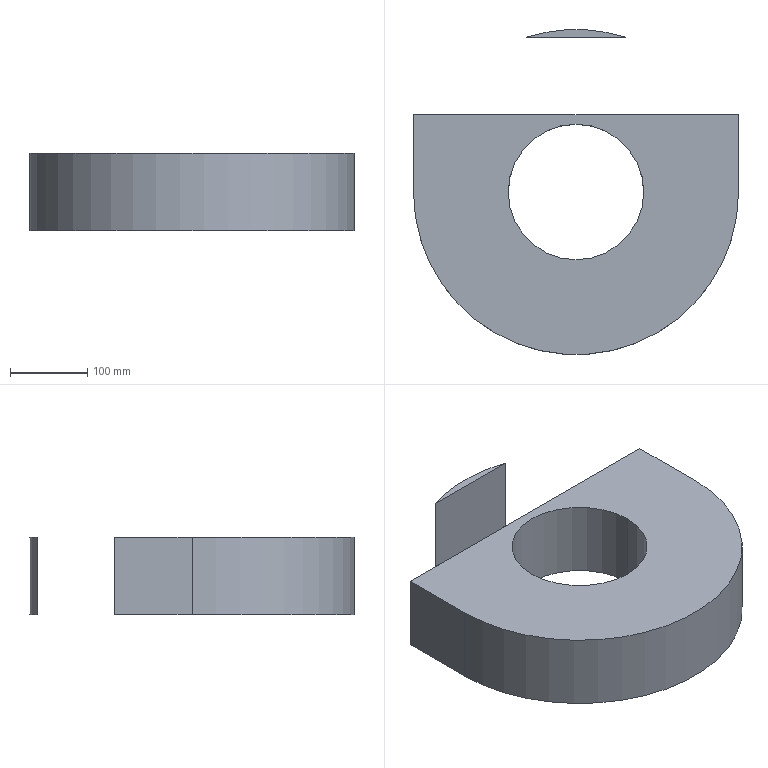Part | SolidWorks | features ICE 2, Extrusion 1 | 2 solids | 12 faces | box 420 x 420 x 100 mm | volume 8807720 mm3 | plane 8 | cylinder 4 | commonest cylinder face diameters 175 x2 420 x2
STEP:
#1=CARTESIAN_POINT('',(-87.5,0.,100.));
#2=VERTEX_POINT('',#1);
#3=CARTESIAN_POINT('',(87.5,0.,100.));
#4=VERTEX_POINT('',#3);
#5=CARTESIAN_POINT('',(0.,0.,100.));
#6=DIRECTION('',(0.,0.,1.));
#7=DIRECTION('',(1.,0.,0.));
#8=AXIS2_PLACEMENT_3D('',#5,#6,#7);
#9=CIRCLE('',#8,87.5);
#10=EDGE_CURVE('',#2,#4,#9,.T.);
#11=ORIENTED_EDGE('',*,*,#10,.T.);
#12=CARTESIAN_POINT('',(87.5,0.,0.));
#13=VERTEX_POINT('',#12);
#14=CARTESIAN_POINT('',(87.5,0.,100.));
#15=DIRECTION('',(0.,0.,-1.));
#16=VECTOR('',#15,1000.);
#17=LINE('',#14,#16);
#18=EDGE_CURVE('',#4,#13,#17,.T.);
#19=ORIENTED_EDGE('',*,*,#18,.T.);
#20=CARTESIAN_POINT('',(-87.5,0.,0.));
#21=VERTEX_POINT('',#20);
#22=CARTESIAN_POINT('',(0.,0.,0.));
#23=DIRECTION('',(0.,0.,1.));
#24=DIRECTION('',(1.,0.,0.));
#25=AXIS2_PLACEMENT_3D('',#22,#23,#24);
#26=CIRCLE('',#25,87.5);
#27=EDGE_CURVE('',#21,#13,#26,.T.);
#28=ORIENTED_EDGE('',*,*,#27,.F.);
#29=CARTESIAN_POINT('',(-87.5,0.,100.));
#30=DIRECTION('',(0.,0.,-1.));
#31=VECTOR('',#30,1000.);
#32=LINE('',#29,#31);
#33=EDGE_CURVE('',#2,#21,#32,.T.);
#34=ORIENTED_EDGE('',*,*,#33,.F.);
#35=EDGE_LOOP('',(#11,#19,#28,#34));
#36=FACE_OUTER_BOUND('',#35,.T.);
#37=CARTESIAN_POINT('',(0.,0.,100.));
#38=DIRECTION('',(0.,0.,-1.));
#39=DIRECTION('',(-1.,0.,0.));
#40=AXIS2_PLACEMENT_3D('',#37,#38,#39);
#41=CYLINDRICAL_SURFACE('',#40,87.5);
#42=ADVANCED_FACE('',(#36),#41,.F.);
#43=CARTESIAN_POINT('',(210.,100.,100.));
#44=VERTEX_POINT('',#43);
#45=CARTESIAN_POINT('',(-210.,100.,100.));
#46=VERTEX_POINT('',#45);
#47=CARTESIAN_POINT('',(184.662,100.,100.));
#48=DIRECTION('',(-1.,0.,0.));
#49=VECTOR('',#48,1000.);
#50=LINE('',#47,#49);
#51=EDGE_CURVE('',#44,#46,#50,.T.);
#52=ORIENTED_EDGE('',*,*,#51,.T.);
#53=CARTESIAN_POINT('',(-210.,0.,100.));
#54=VERTEX_POINT('',#53);
#55=CARTESIAN_POINT('',(-210.,0.,100.));
#56=DIRECTION('',(0.,-1.,0.));
#57=VECTOR('',#56,1000.);
#58=LINE('',#55,#57);
#59=EDGE_CURVE('',#46,#54,#58,.T.);
#60=ORIENTED_EDGE('',*,*,#59,.T.);
#61=CARTESIAN_POINT('',(210.,0.,100.));
#62=VERTEX_POINT('',#61);
#63=CARTESIAN_POINT('',(0.,0.,100.));
#64=DIRECTION('',(0.,0.,1.));
#65=DIRECTION('',(1.,0.,0.));
#66=AXIS2_PLACEMENT_3D('',#63,#64,#65);
#67=CIRCLE('',#66,210.);
#68=EDGE_CURVE('',#54,#62,#67,.T.);
#69=ORIENTED_EDGE('',*,*,#68,.T.);
#70=CARTESIAN_POINT('',(210.,0.,100.));
#71=DIRECTION('',(0.,1.,0.));
#72=VECTOR('',#71,1000.);
#73=LINE('',#70,#72);
#74=EDGE_CURVE('',#62,#44,#73,.T.);
#75=ORIENTED_EDGE('',*,*,#74,.T.);
#76=EDGE_LOOP('',(#52,#60,#69,#75));
#77=FACE_OUTER_BOUND('',#76,.T.);
#78=ORIENTED_EDGE('',*,*,#10,.F.);
#79=CARTESIAN_POINT('',(0.,0.,100.));
#80=DIRECTION('',(0.,0.,1.));
#81=DIRECTION('',(1.,0.,0.));
#82=AXIS2_PLACEMENT_3D('',#79,#80,#81);
#83=CIRCLE('',#82,87.5);
#84=EDGE_CURVE('',#4,#2,#83,.T.);
#85=ORIENTED_EDGE('',*,*,#84,.F.);
#86=EDGE_LOOP('',(#78,#85));
#87=FACE_BOUND('',#86,.T.);
#88=CARTESIAN_POINT('',(0.,0.,100.));
#89=DIRECTION('',(0.,0.,1.));
#90=DIRECTION('',(1.,0.,0.));
#91=AXIS2_PLACEMENT_3D('',#88,#89,#90);
#92=PLANE('',#91);
#93=ADVANCED_FACE('',(#77,#87),#92,.T.);
#94=CARTESIAN_POINT('',(-210.,100.,0.));
#95=VERTEX_POINT('',#94);
#96=CARTESIAN_POINT('',(210.,100.,0.));
#97=VERTEX_POINT('',#96);
#98=CARTESIAN_POINT('',(-210.,100.,0.));
#99=DIRECTION('',(1.,0.,0.));
#100=VECTOR('',#99,1000.);
#101=LINE('',#98,#100);
#102=EDGE_CURVE('',#95,#97,#101,.T.);
#103=ORIENTED_EDGE('',*,*,#102,.T.);
#104=CARTESIAN_POINT('',(210.,0.,0.));
#105=VERTEX_POINT('',#104);
#106=CARTESIAN_POINT('',(210.,0.,0.));
#107=DIRECTION('',(0.,-1.,0.));
#108=VECTOR('',#107,1000.);
#109=LINE('',#106,#108);
#110=EDGE_CURVE('',#97,#105,#109,.T.);
#111=ORIENTED_EDGE('',*,*,#110,.T.);
#112=CARTESIAN_POINT('',(-210.,0.,0.));
#113=VERTEX_POINT('',#112);
#114=CARTESIAN_POINT('',(0.,0.,0.));
#115=DIRECTION('',(0.,0.,1.));
#116=DIRECTION('',(1.,0.,0.));
#117=AXIS2_PLACEMENT_3D('',#114,#115,#116);
#118=CIRCLE('',#117,210.);
#119=EDGE_CURVE('',#113,#105,#118,.T.);
#120=ORIENTED_EDGE('',*,*,#119,.F.);
#121=CARTESIAN_POINT('',(-210.,0.,0.));
#122=DIRECTION('',(0.,1.,0.));
#123=VECTOR('',#122,1000.);
#124=LINE('',#121,#123);
#125=EDGE_CURVE('',#113,#95,#124,.T.);
#126=ORIENTED_EDGE('',*,*,#125,.T.);
#127=EDGE_LOOP('',(#103,#111,#120,#126));
#128=FACE_OUTER_BOUND('',#127,.T.);
#129=ORIENTED_EDGE('',*,*,#27,.T.);
#130=CARTESIAN_POINT('',(0.,0.,0.));
#131=DIRECTION('',(0.,0.,1.));
#132=DIRECTION('',(1.,0.,0.));
#133=AXIS2_PLACEMENT_3D('',#130,#131,#132);
#134=CIRCLE('',#133,87.5);
#135=EDGE_CURVE('',#13,#21,#134,.T.);
#136=ORIENTED_EDGE('',*,*,#135,.T.);
#137=EDGE_LOOP('',(#129,#136));
#138=FACE_BOUND('',#137,.T.);
#139=CARTESIAN_POINT('',(0.,0.,0.));
#140=DIRECTION('',(0.,0.,1.));
#141=DIRECTION('',(1.,0.,0.));
#142=AXIS2_PLACEMENT_3D('',#139,#140,#141);
#143=PLANE('',#142);
#144=ADVANCED_FACE('',(#128,#138),#143,.F.);
#145=ORIENTED_EDGE('',*,*,#119,.T.);
#146=CARTESIAN_POINT('',(210.,0.,-431.741));
#147=DIRECTION('',(0.,0.,1.));
#148=VECTOR('',#147,1000.);
#149=LINE('',#146,#148);
#150=EDGE_CURVE('',#105,#62,#149,.T.);
#151=ORIENTED_EDGE('',*,*,#150,.T.);
#152=ORIENTED_EDGE('',*,*,#68,.F.);
#153=CARTESIAN_POINT('',(-210.,0.,-431.741));
#154=DIRECTION('',(0.,0.,1.));
#155=VECTOR('',#154,1000.);
#156=LINE('',#153,#155);
#157=EDGE_CURVE('',#113,#54,#156,.T.);
#158=ORIENTED_EDGE('',*,*,#157,.F.);
#159=EDGE_LOOP('',(#145,#151,#152,#158));
#160=FACE_OUTER_BOUND('',#159,.T.);
#161=CARTESIAN_POINT('',(0.,0.,100.));
#162=DIRECTION('',(0.,0.,-1.));
#163=DIRECTION('',(-1.,0.,0.));
#164=AXIS2_PLACEMENT_3D('',#161,#162,#163);
#165=CYLINDRICAL_SURFACE('',#164,210.);
#166=ADVANCED_FACE('',(#160),#165,.T.);
#167=ORIENTED_EDGE('',*,*,#18,.F.);
#168=ORIENTED_EDGE('',*,*,#84,.T.);
#169=ORIENTED_EDGE('',*,*,#33,.T.);
#170=ORIENTED_EDGE('',*,*,#135,.F.);
#171=EDGE_LOOP('',(#167,#168,#169,#170));
#172=FACE_OUTER_BOUND('',#171,.T.);
#173=CARTESIAN_POINT('',(0.,0.,100.));
#174=DIRECTION('',(0.,0.,-1.));
#175=DIRECTION('',(-1.,0.,0.));
#176=AXIS2_PLACEMENT_3D('',#173,#174,#175);
#177=CYLINDRICAL_SURFACE('',#176,87.5);
#178=ADVANCED_FACE('',(#172),#177,.F.);
#179=ORIENTED_EDGE('',*,*,#125,.F.);
#180=ORIENTED_EDGE('',*,*,#157,.T.);
#181=ORIENTED_EDGE('',*,*,#59,.F.);
#182=CARTESIAN_POINT('',(-210.,100.,-431.741));
#183=DIRECTION('',(0.,0.,1.));
#184=VECTOR('',#183,1000.);
#185=LINE('',#182,#184);
#186=EDGE_CURVE('',#95,#46,#185,.T.);
#187=ORIENTED_EDGE('',*,*,#186,.F.);
#188=EDGE_LOOP('',(#179,#180,#181,#187));
#189=FACE_OUTER_BOUND('',#188,.T.);
#190=CARTESIAN_POINT('',(-210.,0.,-431.741));
#191=DIRECTION('',(-1.,0.,0.));
#192=DIRECTION('',(0.,0.,1.));
#193=AXIS2_PLACEMENT_3D('',#190,#191,#192);
#194=PLANE('',#193);
#195=ADVANCED_FACE('',(#189),#194,.T.);
#196=ORIENTED_EDGE('',*,*,#186,.T.);
#197=ORIENTED_EDGE('',*,*,#51,.F.);
#198=CARTESIAN_POINT('',(210.,100.,-431.741));
#199=DIRECTION('',(0.,0.,1.));
#200=VECTOR('',#199,1000.);
#201=LINE('',#198,#200);
#202=EDGE_CURVE('',#97,#44,#201,.T.);
#203=ORIENTED_EDGE('',*,*,#202,.F.);
#204=ORIENTED_EDGE('',*,*,#102,.F.);
#205=EDGE_LOOP('',(#196,#197,#203,#204));
#206=FACE_OUTER_BOUND('',#205,.T.);
#207=CARTESIAN_POINT('',(-210.,100.,-431.741));
#208=DIRECTION('',(0.,1.,0.));
#209=DIRECTION('',(0.,0.,1.));
#210=AXIS2_PLACEMENT_3D('',#207,#208,#209);
#211=PLANE('',#210);
#212=ADVANCED_FACE('',(#206),#211,.T.);
#213=ORIENTED_EDGE('',*,*,#110,.F.);
#214=ORIENTED_EDGE('',*,*,#202,.T.);
#215=ORIENTED_EDGE('',*,*,#74,.F.);
#216=ORIENTED_EDGE('',*,*,#150,.F.);
#217=EDGE_LOOP('',(#213,#214,#215,#216));
#218=FACE_OUTER_BOUND('',#217,.T.);
#219=CARTESIAN_POINT('',(210.,0.,-431.741));
#220=DIRECTION('',(1.,0.,0.));
#221=DIRECTION('',(0.,0.,-1.));
#222=AXIS2_PLACEMENT_3D('',#219,#220,#221);
#223=PLANE('',#222);
#224=ADVANCED_FACE('',(#218),#223,.T.);
#225=CLOSED_SHELL('',(#42,#93,#144,#166,#178,#195,#212,#224));
#226=MANIFOLD_SOLID_BREP('',#225);
#227=CARTESIAN_POINT('',(64.031,200.,0.));
#228=VERTEX_POINT('',#227);
#229=CARTESIAN_POINT('',(-64.031,200.,0.));
#230=VERTEX_POINT('',#229);
#231=CARTESIAN_POINT('',(0.,0.,0.));
#232=DIRECTION('',(0.,0.,1.));
#233=DIRECTION('',(1.,0.,0.));
#234=AXIS2_PLACEMENT_3D('',#231,#232,#233);
#235=CIRCLE('',#234,210.);
#236=EDGE_CURVE('',#228,#230,#235,.T.);
#237=ORIENTED_EDGE('',*,*,#236,.F.);
#238=CARTESIAN_POINT('',(0.,200.,0.));
#239=DIRECTION('',(-1.,0.,0.));
#240=VECTOR('',#239,1000.);
#241=LINE('',#238,#240);
#242=EDGE_CURVE('',#228,#230,#241,.T.);
#243=ORIENTED_EDGE('',*,*,#242,.T.);
#244=EDGE_LOOP('',(#237,#243));
#245=FACE_OUTER_BOUND('',#244,.T.);
#246=CARTESIAN_POINT('',(0.,0.,0.));
#247=DIRECTION('',(0.,0.,1.));
#248=DIRECTION('',(1.,0.,0.));
#249=AXIS2_PLACEMENT_3D('',#246,#247,#248);
#250=PLANE('',#249);
#251=ADVANCED_FACE('',(#245),#250,.F.);
#252=CARTESIAN_POINT('',(-64.031,200.,100.));
#253=VERTEX_POINT('',#252);
#254=CARTESIAN_POINT('',(64.031,200.,100.));
#255=VERTEX_POINT('',#254);
#256=CARTESIAN_POINT('',(184.662,200.,100.));
#257=DIRECTION('',(1.,0.,0.));
#258=VECTOR('',#257,1000.);
#259=LINE('',#256,#258);
#260=EDGE_CURVE('',#253,#255,#259,.T.);
#261=ORIENTED_EDGE('',*,*,#260,.T.);
#262=CARTESIAN_POINT('',(0.,0.,100.));
#263=DIRECTION('',(0.,0.,1.));
#264=DIRECTION('',(1.,0.,0.));
#265=AXIS2_PLACEMENT_3D('',#262,#263,#264);
#266=CIRCLE('',#265,210.);
#267=EDGE_CURVE('',#255,#253,#266,.T.);
#268=ORIENTED_EDGE('',*,*,#267,.T.);
#269=EDGE_LOOP('',(#261,#268));
#270=FACE_OUTER_BOUND('',#269,.T.);
#271=CARTESIAN_POINT('',(0.,0.,100.));
#272=DIRECTION('',(0.,0.,1.));
#273=DIRECTION('',(1.,0.,0.));
#274=AXIS2_PLACEMENT_3D('',#271,#272,#273);
#275=PLANE('',#274);
#276=ADVANCED_FACE('',(#270),#275,.T.);
#277=ORIENTED_EDGE('',*,*,#267,.F.);
#278=CARTESIAN_POINT('',(64.031,200.,100.));
#279=DIRECTION('',(0.,0.,-1.));
#280=VECTOR('',#279,1000.);
#281=LINE('',#278,#280);
#282=EDGE_CURVE('',#255,#228,#281,.T.);
#283=ORIENTED_EDGE('',*,*,#282,.T.);
#284=ORIENTED_EDGE('',*,*,#236,.T.);
#285=CARTESIAN_POINT('',(-64.031,200.,100.));
#286=DIRECTION('',(0.,0.,1.));
#287=VECTOR('',#286,1000.);
#288=LINE('',#285,#287);
#289=EDGE_CURVE('',#230,#253,#288,.T.);
#290=ORIENTED_EDGE('',*,*,#289,.T.);
#291=EDGE_LOOP('',(#277,#283,#284,#290));
#292=FACE_OUTER_BOUND('',#291,.T.);
#293=CARTESIAN_POINT('',(0.,0.,100.));
#294=DIRECTION('',(0.,0.,-1.));
#295=DIRECTION('',(-1.,0.,0.));
#296=AXIS2_PLACEMENT_3D('',#293,#294,#295);
#297=CYLINDRICAL_SURFACE('',#296,210.);
#298=ADVANCED_FACE('',(#292),#297,.T.);
#299=ORIENTED_EDGE('',*,*,#260,.F.);
#300=ORIENTED_EDGE('',*,*,#289,.F.);
#301=ORIENTED_EDGE('',*,*,#242,.F.);
#302=ORIENTED_EDGE('',*,*,#282,.F.);
#303=EDGE_LOOP('',(#299,#300,#301,#302));
#304=FACE_OUTER_BOUND('',#303,.T.);
#305=CARTESIAN_POINT('',(184.662,200.,100.));
#306=DIRECTION('',(0.,1.,0.));
#307=DIRECTION('',(0.,0.,1.));
#308=AXIS2_PLACEMENT_3D('',#305,#306,#307);
#309=PLANE('',#308);
#310=ADVANCED_FACE('',(#304),#309,.F.);
#311=CLOSED_SHELL('',(#251,#276,#298,#310));
#312=MANIFOLD_SOLID_BREP('',#311);
#313=CARTESIAN_POINT('',(0.,0.,0.));
#314=DIRECTION('',(0.,0.,1.));
#315=DIRECTION('',(1.,0.,0.));
#316=AXIS2_PLACEMENT_3D('',#313,#314,#315);
#317=(LENGTH_UNIT()NAMED_UNIT(*)SI_UNIT(.MILLI.,.METRE.));
#318=UNCERTAINTY_MEASURE_WITH_UNIT(LENGTH_MEASURE(0.00001),#317,'','');
#319=(NAMED_UNIT(*)PLANE_ANGLE_UNIT()SI_UNIT($,.RADIAN.));
#320=(NAMED_UNIT(*)SI_UNIT($,.STERADIAN.)SOLID_ANGLE_UNIT());
#321=(GEOMETRIC_REPRESENTATION_CONTEXT(3)GLOBAL_UNCERTAINTY_ASSIGNED_CONTEXT((#318))GLOBAL_UNIT_ASSIGNED_CONTEXT((#317,#319,#320))REPRESENTATION_CONTEXT('',''));
#322=ADVANCED_BREP_SHAPE_REPRESENTATION('',(#226,#312,#316),#321);